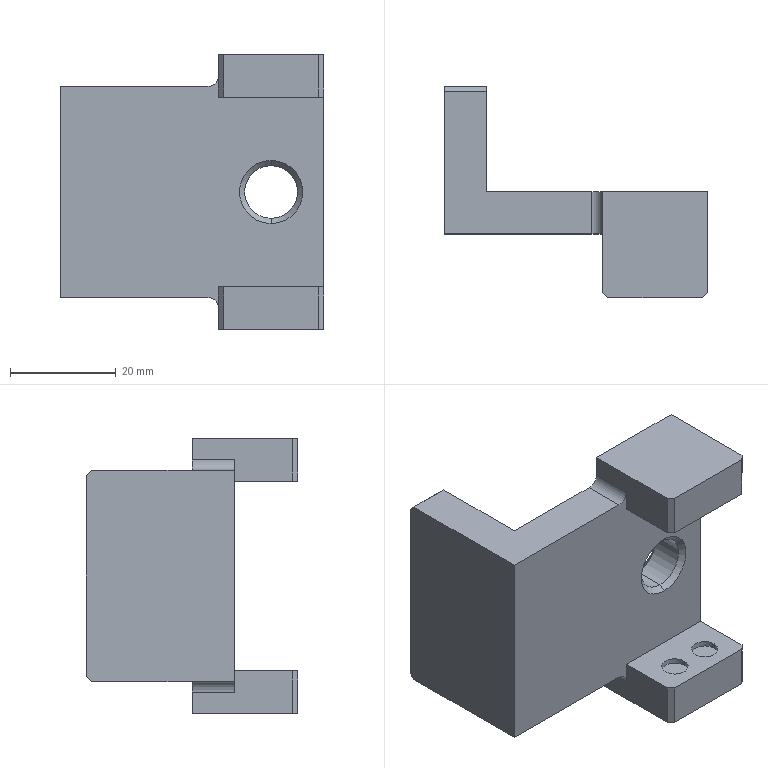Part | SolidWorks | features ICE 5, Chamfer 3, Cut 1, Extrusion 1, Fillet 1 | 1 solid | 42 faces | box 50 x 40 x 52 mm | volume 27409 mm3 | plane 26 | cylinder 12 | cone 4 | commonest cylinder face diameters 5 x8 4 x2 10 x2
STEP:
#1=CARTESIAN_POINT('',(38.5,-7.,39.));
#2=VERTEX_POINT('',#1);
#3=CARTESIAN_POINT('',(33.5,-7.,39.));
#4=VERTEX_POINT('',#3);
#5=CARTESIAN_POINT('',(36.,-7.,39.));
#6=DIRECTION('',(0.,0.,-1.));
#7=DIRECTION('',(-1.,0.,0.));
#8=AXIS2_PLACEMENT_3D('',#5,#6,#7);
#9=CIRCLE('',#8,2.5);
#10=EDGE_CURVE('',#2,#4,#9,.T.);
#11=ORIENTED_EDGE('',*,*,#10,.F.);
#12=CARTESIAN_POINT('',(38.5,-7.,38.));
#13=VERTEX_POINT('',#12);
#14=CARTESIAN_POINT('',(38.5,-7.,39.));
#15=DIRECTION('',(0.,0.,-1.));
#16=VECTOR('',#15,1000.);
#17=LINE('',#14,#16);
#18=EDGE_CURVE('',#2,#13,#17,.T.);
#19=ORIENTED_EDGE('',*,*,#18,.T.);
#20=CARTESIAN_POINT('',(33.5,-7.,38.));
#21=VERTEX_POINT('',#20);
#22=CARTESIAN_POINT('',(36.,-7.,38.));
#23=DIRECTION('',(0.,0.,-1.));
#24=DIRECTION('',(-1.,0.,0.));
#25=AXIS2_PLACEMENT_3D('',#22,#23,#24);
#26=CIRCLE('',#25,2.5);
#27=EDGE_CURVE('',#13,#21,#26,.T.);
#28=ORIENTED_EDGE('',*,*,#27,.T.);
#29=CARTESIAN_POINT('',(33.5,-7.,39.));
#30=DIRECTION('',(0.,0.,-1.));
#31=VECTOR('',#30,1000.);
#32=LINE('',#29,#31);
#33=EDGE_CURVE('',#4,#21,#32,.T.);
#34=ORIENTED_EDGE('',*,*,#33,.F.);
#35=EDGE_LOOP('',(#11,#19,#28,#34));
#36=FACE_OUTER_BOUND('',#35,.T.);
#37=CARTESIAN_POINT('',(36.,-7.,39.));
#38=DIRECTION('',(0.,0.,-1.));
#39=DIRECTION('',(-1.,0.,0.));
#40=AXIS2_PLACEMENT_3D('',#37,#38,#39);
#41=CYLINDRICAL_SURFACE('',#40,2.5);
#42=ADVANCED_FACE('',(#36),#41,.F.);
#43=CARTESIAN_POINT('',(46.5,-7.,39.));
#44=VERTEX_POINT('',#43);
#45=CARTESIAN_POINT('',(41.5,-7.,39.));
#46=VERTEX_POINT('',#45);
#47=CARTESIAN_POINT('',(44.,-7.,39.));
#48=DIRECTION('',(0.,0.,-1.));
#49=DIRECTION('',(-1.,0.,0.));
#50=AXIS2_PLACEMENT_3D('',#47,#48,#49);
#51=CIRCLE('',#50,2.5);
#52=EDGE_CURVE('',#44,#46,#51,.T.);
#53=ORIENTED_EDGE('',*,*,#52,.F.);
#54=CARTESIAN_POINT('',(46.5,-7.,38.));
#55=VERTEX_POINT('',#54);
#56=CARTESIAN_POINT('',(46.5,-7.,39.));
#57=DIRECTION('',(0.,0.,-1.));
#58=VECTOR('',#57,1000.);
#59=LINE('',#56,#58);
#60=EDGE_CURVE('',#44,#55,#59,.T.);
#61=ORIENTED_EDGE('',*,*,#60,.T.);
#62=CARTESIAN_POINT('',(41.5,-7.,38.));
#63=VERTEX_POINT('',#62);
#64=CARTESIAN_POINT('',(44.,-7.,38.));
#65=DIRECTION('',(0.,0.,-1.));
#66=DIRECTION('',(-1.,0.,0.));
#67=AXIS2_PLACEMENT_3D('',#64,#65,#66);
#68=CIRCLE('',#67,2.5);
#69=EDGE_CURVE('',#55,#63,#68,.T.);
#70=ORIENTED_EDGE('',*,*,#69,.T.);
#71=CARTESIAN_POINT('',(41.5,-7.,39.));
#72=DIRECTION('',(0.,0.,-1.));
#73=VECTOR('',#72,1000.);
#74=LINE('',#71,#73);
#75=EDGE_CURVE('',#46,#63,#74,.T.);
#76=ORIENTED_EDGE('',*,*,#75,.F.);
#77=EDGE_LOOP('',(#53,#61,#70,#76));
#78=FACE_OUTER_BOUND('',#77,.T.);
#79=CARTESIAN_POINT('',(44.,-7.,39.));
#80=DIRECTION('',(0.,0.,-1.));
#81=DIRECTION('',(-1.,0.,0.));
#82=AXIS2_PLACEMENT_3D('',#79,#80,#81);
#83=CYLINDRICAL_SURFACE('',#82,2.5);
#84=ADVANCED_FACE('',(#78),#83,.F.);
#85=CARTESIAN_POINT('',(41.5,-7.,1.));
#86=VERTEX_POINT('',#85);
#87=CARTESIAN_POINT('',(46.5,-7.,1.));
#88=VERTEX_POINT('',#87);
#89=CARTESIAN_POINT('',(44.,-7.,1.));
#90=DIRECTION('',(0.,0.,1.));
#91=DIRECTION('',(1.,0.,0.));
#92=AXIS2_PLACEMENT_3D('',#89,#90,#91);
#93=CIRCLE('',#92,2.5);
#94=EDGE_CURVE('',#86,#88,#93,.T.);
#95=ORIENTED_EDGE('',*,*,#94,.F.);
#96=CARTESIAN_POINT('',(41.5,-7.,2.));
#97=VERTEX_POINT('',#96);
#98=CARTESIAN_POINT('',(41.5,-7.,1.));
#99=DIRECTION('',(0.,0.,1.));
#100=VECTOR('',#99,1000.);
#101=LINE('',#98,#100);
#102=EDGE_CURVE('',#86,#97,#101,.T.);
#103=ORIENTED_EDGE('',*,*,#102,.T.);
#104=CARTESIAN_POINT('',(46.5,-7.,2.));
#105=VERTEX_POINT('',#104);
#106=CARTESIAN_POINT('',(44.,-7.,2.));
#107=DIRECTION('',(0.,0.,1.));
#108=DIRECTION('',(1.,0.,0.));
#109=AXIS2_PLACEMENT_3D('',#106,#107,#108);
#110=CIRCLE('',#109,2.5);
#111=EDGE_CURVE('',#97,#105,#110,.T.);
#112=ORIENTED_EDGE('',*,*,#111,.T.);
#113=CARTESIAN_POINT('',(46.5,-7.,1.));
#114=DIRECTION('',(0.,0.,1.));
#115=VECTOR('',#114,1000.);
#116=LINE('',#113,#115);
#117=EDGE_CURVE('',#88,#105,#116,.T.);
#118=ORIENTED_EDGE('',*,*,#117,.F.);
#119=EDGE_LOOP('',(#95,#103,#112,#118));
#120=FACE_OUTER_BOUND('',#119,.T.);
#121=CARTESIAN_POINT('',(44.,-7.,1.));
#122=DIRECTION('',(0.,0.,1.));
#123=DIRECTION('',(1.,0.,0.));
#124=AXIS2_PLACEMENT_3D('',#121,#122,#123);
#125=CYLINDRICAL_SURFACE('',#124,2.5);
#126=ADVANCED_FACE('',(#120),#125,.F.);
#127=CARTESIAN_POINT('',(33.5,-7.,1.));
#128=VERTEX_POINT('',#127);
#129=CARTESIAN_POINT('',(38.5,-7.,1.));
#130=VERTEX_POINT('',#129);
#131=CARTESIAN_POINT('',(36.,-7.,1.));
#132=DIRECTION('',(0.,0.,1.));
#133=DIRECTION('',(1.,0.,0.));
#134=AXIS2_PLACEMENT_3D('',#131,#132,#133);
#135=CIRCLE('',#134,2.5);
#136=EDGE_CURVE('',#128,#130,#135,.T.);
#137=ORIENTED_EDGE('',*,*,#136,.F.);
#138=CARTESIAN_POINT('',(33.5,-7.,2.));
#139=VERTEX_POINT('',#138);
#140=CARTESIAN_POINT('',(33.5,-7.,1.));
#141=DIRECTION('',(0.,0.,1.));
#142=VECTOR('',#141,1000.);
#143=LINE('',#140,#142);
#144=EDGE_CURVE('',#128,#139,#143,.T.);
#145=ORIENTED_EDGE('',*,*,#144,.T.);
#146=CARTESIAN_POINT('',(38.5,-7.,2.));
#147=VERTEX_POINT('',#146);
#148=CARTESIAN_POINT('',(36.,-7.,2.));
#149=DIRECTION('',(0.,0.,1.));
#150=DIRECTION('',(1.,0.,0.));
#151=AXIS2_PLACEMENT_3D('',#148,#149,#150);
#152=CIRCLE('',#151,2.5);
#153=EDGE_CURVE('',#139,#147,#152,.T.);
#154=ORIENTED_EDGE('',*,*,#153,.T.);
#155=CARTESIAN_POINT('',(38.5,-7.,1.));
#156=DIRECTION('',(0.,0.,1.));
#157=VECTOR('',#156,1000.);
#158=LINE('',#155,#157);
#159=EDGE_CURVE('',#130,#147,#158,.T.);
#160=ORIENTED_EDGE('',*,*,#159,.F.);
#161=EDGE_LOOP('',(#137,#145,#154,#160));
#162=FACE_OUTER_BOUND('',#161,.T.);
#163=CARTESIAN_POINT('',(36.,-7.,1.));
#164=DIRECTION('',(0.,0.,1.));
#165=DIRECTION('',(1.,0.,0.));
#166=AXIS2_PLACEMENT_3D('',#163,#164,#165);
#167=CYLINDRICAL_SURFACE('',#166,2.5);
#168=ADVANCED_FACE('',(#162),#167,.F.);
#169=CARTESIAN_POINT('',(40.,1.,25.));
#170=VERTEX_POINT('',#169);
#171=CARTESIAN_POINT('',(40.,1.,15.));
#172=VERTEX_POINT('',#171);
#173=CARTESIAN_POINT('',(40.,1.,20.));
#174=DIRECTION('',(0.,-1.,0.));
#175=DIRECTION('',(0.,0.,1.));
#176=AXIS2_PLACEMENT_3D('',#173,#174,#175);
#177=CIRCLE('',#176,5.);
#178=EDGE_CURVE('',#170,#172,#177,.T.);
#179=ORIENTED_EDGE('',*,*,#178,.F.);
#180=CARTESIAN_POINT('',(40.,0.,26.));
#181=VERTEX_POINT('',#180);
#182=CARTESIAN_POINT('',(40.,1.,25.));
#183=DIRECTION('',(0.,-0.7071,0.7071));
#184=VECTOR('',#183,1000.);
#185=LINE('',#182,#184);
#186=EDGE_CURVE('',#170,#181,#185,.T.);
#187=ORIENTED_EDGE('',*,*,#186,.T.);
#188=CARTESIAN_POINT('',(40.,0.,14.));
#189=VERTEX_POINT('',#188);
#190=CARTESIAN_POINT('',(40.,0.,20.));
#191=DIRECTION('',(0.,1.,0.));
#192=DIRECTION('',(0.,0.,1.));
#193=AXIS2_PLACEMENT_3D('',#190,#191,#192);
#194=CIRCLE('',#193,6.);
#195=EDGE_CURVE('',#189,#181,#194,.T.);
#196=ORIENTED_EDGE('',*,*,#195,.F.);
#197=CARTESIAN_POINT('',(40.,1.,15.));
#198=DIRECTION('',(0.,-0.7071,-0.7071));
#199=VECTOR('',#198,1000.);
#200=LINE('',#197,#199);
#201=EDGE_CURVE('',#172,#189,#200,.T.);
#202=ORIENTED_EDGE('',*,*,#201,.F.);
#203=EDGE_LOOP('',(#179,#187,#196,#202));
#204=FACE_OUTER_BOUND('',#203,.T.);
#205=CARTESIAN_POINT('',(40.,1.,20.));
#206=DIRECTION('',(0.,-1.,0.));
#207=DIRECTION('',(0.,0.,-1.));
#208=AXIS2_PLACEMENT_3D('',#205,#206,#207);
#209=CONICAL_SURFACE('',#208,5.,0.7854);
#210=ADVANCED_FACE('',(#204),#209,.F.);
#211=CARTESIAN_POINT('',(40.,7.,15.));
#212=VERTEX_POINT('',#211);
#213=CARTESIAN_POINT('',(40.,7.,25.));
#214=VERTEX_POINT('',#213);
#215=CARTESIAN_POINT('',(40.,7.,20.));
#216=DIRECTION('',(0.,1.,0.));
#217=DIRECTION('',(0.,0.,1.));
#218=AXIS2_PLACEMENT_3D('',#215,#216,#217);
#219=CIRCLE('',#218,5.);
#220=EDGE_CURVE('',#212,#214,#219,.T.);
#221=ORIENTED_EDGE('',*,*,#220,.F.);
#222=CARTESIAN_POINT('',(40.,8.,14.));
#223=VERTEX_POINT('',#222);
#224=CARTESIAN_POINT('',(40.,8.,14.));
#225=DIRECTION('',(0.,0.7071,-0.7071));
#226=VECTOR('',#225,1000.);
#227=LINE('',#224,#226);
#228=EDGE_CURVE('',#212,#223,#227,.T.);
#229=ORIENTED_EDGE('',*,*,#228,.T.);
#230=CARTESIAN_POINT('',(40.,8.,26.));
#231=VERTEX_POINT('',#230);
#232=CARTESIAN_POINT('',(40.,8.,20.));
#233=DIRECTION('',(0.,-1.,0.));
#234=DIRECTION('',(0.,0.,1.));
#235=AXIS2_PLACEMENT_3D('',#232,#233,#234);
#236=CIRCLE('',#235,6.);
#237=EDGE_CURVE('',#231,#223,#236,.T.);
#238=ORIENTED_EDGE('',*,*,#237,.F.);
#239=CARTESIAN_POINT('',(40.,8.,26.));
#240=DIRECTION('',(0.,0.7071,0.7071));
#241=VECTOR('',#240,1000.);
#242=LINE('',#239,#241);
#243=EDGE_CURVE('',#214,#231,#242,.T.);
#244=ORIENTED_EDGE('',*,*,#243,.F.);
#245=EDGE_LOOP('',(#221,#229,#238,#244));
#246=FACE_OUTER_BOUND('',#245,.T.);
#247=CARTESIAN_POINT('',(40.,8.,20.));
#248=DIRECTION('',(0.,1.,0.));
#249=DIRECTION('',(0.,0.,1.));
#250=AXIS2_PLACEMENT_3D('',#247,#248,#249);
#251=CONICAL_SURFACE('',#250,6.,0.7854);
#252=ADVANCED_FACE('',(#246),#251,.F.);
#253=ORIENTED_EDGE('',*,*,#220,.T.);
#254=CARTESIAN_POINT('',(40.,8.,25.));
#255=DIRECTION('',(0.,-1.,0.));
#256=VECTOR('',#255,1000.);
#257=LINE('',#254,#256);
#258=EDGE_CURVE('',#214,#170,#257,.T.);
#259=ORIENTED_EDGE('',*,*,#258,.T.);
#260=ORIENTED_EDGE('',*,*,#178,.T.);
#261=CARTESIAN_POINT('',(40.,8.,15.));
#262=DIRECTION('',(0.,-1.,0.));
#263=VECTOR('',#262,1000.);
#264=LINE('',#261,#263);
#265=EDGE_CURVE('',#212,#172,#264,.T.);
#266=ORIENTED_EDGE('',*,*,#265,.F.);
#267=EDGE_LOOP('',(#253,#259,#260,#266));
#268=FACE_OUTER_BOUND('',#267,.T.);
#269=CARTESIAN_POINT('',(40.,8.,20.));
#270=DIRECTION('',(0.,-1.,0.));
#271=DIRECTION('',(0.,0.,-1.));
#272=AXIS2_PLACEMENT_3D('',#269,#270,#271);
#273=CYLINDRICAL_SURFACE('',#272,5.);
#274=ADVANCED_FACE('',(#268),#273,.F.);
#275=CARTESIAN_POINT('',(0.,28.,1.));
#276=VERTEX_POINT('',#275);
#277=CARTESIAN_POINT('',(0.,28.,39.));
#278=VERTEX_POINT('',#277);
#279=CARTESIAN_POINT('',(0.,28.,0.));
#280=DIRECTION('',(0.,0.,1.));
#281=VECTOR('',#280,1000.);
#282=LINE('',#279,#281);
#283=EDGE_CURVE('',#276,#278,#282,.T.);
#284=ORIENTED_EDGE('',*,*,#283,.F.);
#285=CARTESIAN_POINT('',(0.,27.,0.));
#286=VERTEX_POINT('',#285);
#287=CARTESIAN_POINT('',(0.,28.,1.));
#288=DIRECTION('',(0.,-0.7071,-0.7071));
#289=VECTOR('',#288,1000.);
#290=LINE('',#287,#289);
#291=EDGE_CURVE('',#276,#286,#290,.T.);
#292=ORIENTED_EDGE('',*,*,#291,.T.);
#293=CARTESIAN_POINT('',(0.,0.,0.));
#294=VERTEX_POINT('',#293);
#295=CARTESIAN_POINT('',(0.,8.,0.));
#296=DIRECTION('',(0.,-1.,0.));
#297=VECTOR('',#296,1000.);
#298=LINE('',#295,#297);
#299=EDGE_CURVE('',#286,#294,#298,.T.);
#300=ORIENTED_EDGE('',*,*,#299,.T.);
#301=CARTESIAN_POINT('',(0.,0.,40.));
#302=VERTEX_POINT('',#301);
#303=CARTESIAN_POINT('',(0.,0.,0.));
#304=DIRECTION('',(0.,0.,1.));
#305=VECTOR('',#304,1000.);
#306=LINE('',#303,#305);
#307=EDGE_CURVE('',#294,#302,#306,.T.);
#308=ORIENTED_EDGE('',*,*,#307,.T.);
#309=CARTESIAN_POINT('',(0.,27.,40.));
#310=VERTEX_POINT('',#309);
#311=CARTESIAN_POINT('',(0.,8.,40.));
#312=DIRECTION('',(0.,-1.,0.));
#313=VECTOR('',#312,1000.);
#314=LINE('',#311,#313);
#315=EDGE_CURVE('',#310,#302,#314,.T.);
#316=ORIENTED_EDGE('',*,*,#315,.F.);
#317=CARTESIAN_POINT('',(0.,28.,39.));
#318=DIRECTION('',(0.,0.7071,-0.7071));
#319=VECTOR('',#318,1000.);
#320=LINE('',#317,#319);
#321=EDGE_CURVE('',#310,#278,#320,.T.);
#322=ORIENTED_EDGE('',*,*,#321,.T.);
#323=EDGE_LOOP('',(#284,#292,#300,#308,#316,#322));
#324=FACE_OUTER_BOUND('',#323,.T.);
#325=CARTESIAN_POINT('',(0.,8.,0.));
#326=DIRECTION('',(1.,0.,0.));
#327=DIRECTION('',(0.,0.,-1.));
#328=AXIS2_PLACEMENT_3D('',#325,#326,#327);
#329=PLANE('',#328);
#330=ADVANCED_FACE('',(#324),#329,.F.);
#331=CARTESIAN_POINT('',(8.,27.,40.));
#332=VERTEX_POINT('',#331);
#333=CARTESIAN_POINT('',(8.,8.,40.));
#334=VERTEX_POINT('',#333);
#335=CARTESIAN_POINT('',(8.,28.,40.));
#336=DIRECTION('',(0.,-1.,0.));
#337=VECTOR('',#336,1000.);
#338=LINE('',#335,#337);
#339=EDGE_CURVE('',#332,#334,#338,.T.);
#340=ORIENTED_EDGE('',*,*,#339,.F.);
#341=CARTESIAN_POINT('',(0.,27.,40.));
#342=DIRECTION('',(-1.,0.,0.));
#343=VECTOR('',#342,1000.);
#344=LINE('',#341,#343);
#345=EDGE_CURVE('',#332,#310,#344,.T.);
#346=ORIENTED_EDGE('',*,*,#345,.T.);
#347=ORIENTED_EDGE('',*,*,#315,.T.);
#348=CARTESIAN_POINT('',(28.,0.,40.));
#349=VERTEX_POINT('',#348);
#350=CARTESIAN_POINT('',(0.,0.,40.));
#351=DIRECTION('',(1.,0.,0.));
#352=VECTOR('',#351,1000.);
#353=LINE('',#350,#352);
#354=EDGE_CURVE('',#302,#349,#353,.T.);
#355=ORIENTED_EDGE('',*,*,#354,.T.);
#356=CARTESIAN_POINT('',(28.,8.,40.));
#357=VERTEX_POINT('',#356);
#358=CARTESIAN_POINT('',(28.,8.,40.));
#359=DIRECTION('',(0.,1.,0.));
#360=VECTOR('',#359,1000.);
#361=LINE('',#358,#360);
#362=EDGE_CURVE('',#349,#357,#361,.T.);
#363=ORIENTED_EDGE('',*,*,#362,.T.);
#364=CARTESIAN_POINT('',(0.,8.,40.));
#365=DIRECTION('',(1.,0.,0.));
#366=VECTOR('',#365,1000.);
#367=LINE('',#364,#366);
#368=EDGE_CURVE('',#334,#357,#367,.T.);
#369=ORIENTED_EDGE('',*,*,#368,.F.);
#370=EDGE_LOOP('',(#340,#346,#347,#355,#363,#369));
#371=FACE_OUTER_BOUND('',#370,.T.);
#372=CARTESIAN_POINT('',(0.,8.,40.));
#373=DIRECTION('',(0.,0.,-1.));
#374=DIRECTION('',(-1.,0.,0.));
#375=AXIS2_PLACEMENT_3D('',#372,#373,#374);
#376=PLANE('',#375);
#377=ADVANCED_FACE('',(#371),#376,.F.);
#378=CARTESIAN_POINT('',(50.,-11.,46.));
#379=VERTEX_POINT('',#378);
#380=CARTESIAN_POINT('',(50.,8.,46.));
#381=VERTEX_POINT('',#380);
#382=CARTESIAN_POINT('',(50.,-55.714,46.));
#383=DIRECTION('',(0.,1.,0.));
#384=VECTOR('',#383,1000.);
#385=LINE('',#382,#384);
#386=EDGE_CURVE('',#379,#381,#385,.T.);
#387=ORIENTED_EDGE('',*,*,#386,.F.);
#388=CARTESIAN_POINT('',(50.,-11.,38.));
#389=VERTEX_POINT('',#388);
#390=CARTESIAN_POINT('',(50.,-11.,38.));
#391=DIRECTION('',(0.,0.,-1.));
#392=VECTOR('',#391,1000.);
#393=LINE('',#390,#392);
#394=EDGE_CURVE('',#379,#389,#393,.T.);
#395=ORIENTED_EDGE('',*,*,#394,.T.);
#396=CARTESIAN_POINT('',(50.,0.,38.));
#397=VERTEX_POINT('',#396);
#398=CARTESIAN_POINT('',(50.,-12.,38.));
#399=DIRECTION('',(0.,1.,0.));
#400=VECTOR('',#399,1000.);
#401=LINE('',#398,#400);
#402=EDGE_CURVE('',#389,#397,#401,.T.);
#403=ORIENTED_EDGE('',*,*,#402,.T.);
#404=CARTESIAN_POINT('',(50.,0.,2.));
#405=VERTEX_POINT('',#404);
#406=CARTESIAN_POINT('',(50.,0.,0.));
#407=DIRECTION('',(0.,0.,-1.));
#408=VECTOR('',#407,1000.);
#409=LINE('',#406,#408);
#410=EDGE_CURVE('',#397,#405,#409,.T.);
#411=ORIENTED_EDGE('',*,*,#410,.T.);
#412=CARTESIAN_POINT('',(50.,-11.,2.));
#413=VERTEX_POINT('',#412);
#414=CARTESIAN_POINT('',(50.,-12.,2.));
#415=DIRECTION('',(0.,1.,0.));
#416=VECTOR('',#415,1000.);
#417=LINE('',#414,#416);
#418=EDGE_CURVE('',#413,#405,#417,.T.);
#419=ORIENTED_EDGE('',*,*,#418,.F.);
#420=CARTESIAN_POINT('',(50.,-11.,-6.));
#421=VERTEX_POINT('',#420);
#422=CARTESIAN_POINT('',(50.,-11.,0.));
#423=DIRECTION('',(0.,0.,-1.));
#424=VECTOR('',#423,1000.);
#425=LINE('',#422,#424);
#426=EDGE_CURVE('',#413,#421,#425,.T.);
#427=ORIENTED_EDGE('',*,*,#426,.T.);
#428=CARTESIAN_POINT('',(50.,8.,-6.));
#429=VERTEX_POINT('',#428);
#430=CARTESIAN_POINT('',(50.,-55.714,-6.));
#431=DIRECTION('',(0.,1.,0.));
#432=VECTOR('',#431,1000.);
#433=LINE('',#430,#432);
#434=EDGE_CURVE('',#421,#429,#433,.T.);
#435=ORIENTED_EDGE('',*,*,#434,.T.);
#436=CARTESIAN_POINT('',(50.,8.,0.));
#437=DIRECTION('',(0.,0.,-1.));
#438=VECTOR('',#437,1000.);
#439=LINE('',#436,#438);
#440=EDGE_CURVE('',#381,#429,#439,.T.);
#441=ORIENTED_EDGE('',*,*,#440,.F.);
#442=EDGE_LOOP('',(#387,#395,#403,#411,#419,#427,#435,#441));
#443=FACE_OUTER_BOUND('',#442,.T.);
#444=CARTESIAN_POINT('',(50.,8.,0.));
#445=DIRECTION('',(-1.,0.,0.));
#446=DIRECTION('',(0.,0.,1.));
#447=AXIS2_PLACEMENT_3D('',#444,#445,#446);
#448=PLANE('',#447);
#449=ADVANCED_FACE('',(#443),#448,.F.);
#450=ORIENTED_EDGE('',*,*,#299,.F.);
#451=CARTESIAN_POINT('',(8.,27.,0.));
#452=VERTEX_POINT('',#451);
#453=CARTESIAN_POINT('',(8.,27.,0.));
#454=DIRECTION('',(1.,0.,0.));
#455=VECTOR('',#454,1000.);
#456=LINE('',#453,#455);
#457=EDGE_CURVE('',#286,#452,#456,.T.);
#458=ORIENTED_EDGE('',*,*,#457,.T.);
#459=CARTESIAN_POINT('',(8.,8.,0.));
#460=VERTEX_POINT('',#459);
#461=CARTESIAN_POINT('',(8.,28.,0.));
#462=DIRECTION('',(0.,-1.,0.));
#463=VECTOR('',#462,1000.);
#464=LINE('',#461,#463);
#465=EDGE_CURVE('',#452,#460,#464,.T.);
#466=ORIENTED_EDGE('',*,*,#465,.T.);
#467=CARTESIAN_POINT('',(28.,8.,0.));
#468=VERTEX_POINT('',#467);
#469=CARTESIAN_POINT('',(0.,8.,0.));
#470=DIRECTION('',(-1.,0.,0.));
#471=VECTOR('',#470,1000.);
#472=LINE('',#469,#471);
#473=EDGE_CURVE('',#468,#460,#472,.T.);
#474=ORIENTED_EDGE('',*,*,#473,.F.);
#475=CARTESIAN_POINT('',(28.,0.,0.));
#476=VERTEX_POINT('',#475);
#477=CARTESIAN_POINT('',(28.,8.,0.));
#478=DIRECTION('',(0.,-1.,0.));
#479=VECTOR('',#478,1000.);
#480=LINE('',#477,#479);
#481=EDGE_CURVE('',#468,#476,#480,.T.);
#482=ORIENTED_EDGE('',*,*,#481,.T.);
#483=CARTESIAN_POINT('',(0.,0.,0.));
#484=DIRECTION('',(-1.,0.,0.));
#485=VECTOR('',#484,1000.);
#486=LINE('',#483,#485);
#487=EDGE_CURVE('',#476,#294,#486,.T.);
#488=ORIENTED_EDGE('',*,*,#487,.T.);
#489=EDGE_LOOP('',(#450,#458,#466,#474,#482,#488));
#490=FACE_OUTER_BOUND('',#489,.T.);
#491=CARTESIAN_POINT('',(0.,8.,0.));
#492=DIRECTION('',(0.,0.,1.));
#493=DIRECTION('',(1.,0.,0.));
#494=AXIS2_PLACEMENT_3D('',#491,#492,#493);
#495=PLANE('',#494);
#496=ADVANCED_FACE('',(#490),#495,.F.);
#497=CARTESIAN_POINT('',(8.,8.,0.));
#498=DIRECTION('',(0.,0.,-1.));
#499=VECTOR('',#498,1000.);
#500=LINE('',#497,#499);
#501=EDGE_CURVE('',#334,#460,#500,.T.);
#502=ORIENTED_EDGE('',*,*,#501,.F.);
#503=ORIENTED_EDGE('',*,*,#368,.T.);
#504=CARTESIAN_POINT('',(30.,8.,42.));
#505=VERTEX_POINT('',#504);
#506=CARTESIAN_POINT('',(28.,8.,42.));
#507=DIRECTION('',(0.,-1.,0.));
#508=DIRECTION('',(0.,0.,1.));
#509=AXIS2_PLACEMENT_3D('',#506,#507,#508);
#510=CIRCLE('',#509,2.);
#511=EDGE_CURVE('',#357,#505,#510,.T.);
#512=ORIENTED_EDGE('',*,*,#511,.T.);
#513=CARTESIAN_POINT('',(30.,8.,46.));
#514=VERTEX_POINT('',#513);
#515=CARTESIAN_POINT('',(30.,8.,-6.));
#516=DIRECTION('',(0.,0.,1.));
#517=VECTOR('',#516,1000.);
#518=LINE('',#515,#517);
#519=EDGE_CURVE('',#505,#514,#518,.T.);
#520=ORIENTED_EDGE('',*,*,#519,.T.);
#521=CARTESIAN_POINT('',(30.,8.,46.));
#522=DIRECTION('',(1.,0.,0.));
#523=VECTOR('',#522,1000.);
#524=LINE('',#521,#523);
#525=EDGE_CURVE('',#514,#381,#524,.T.);
#526=ORIENTED_EDGE('',*,*,#525,.T.);
#527=ORIENTED_EDGE('',*,*,#440,.T.);
#528=CARTESIAN_POINT('',(30.,8.,-6.));
#529=VERTEX_POINT('',#528);
#530=CARTESIAN_POINT('',(30.,8.,-6.));
#531=DIRECTION('',(-1.,0.,0.));
#532=VECTOR('',#531,1000.);
#533=LINE('',#530,#532);
#534=EDGE_CURVE('',#429,#529,#533,.T.);
#535=ORIENTED_EDGE('',*,*,#534,.T.);
#536=CARTESIAN_POINT('',(30.,8.,-2.));
#537=VERTEX_POINT('',#536);
#538=CARTESIAN_POINT('',(30.,8.,-6.));
#539=DIRECTION('',(0.,0.,1.));
#540=VECTOR('',#539,1000.);
#541=LINE('',#538,#540);
#542=EDGE_CURVE('',#529,#537,#541,.T.);
#543=ORIENTED_EDGE('',*,*,#542,.T.);
#544=CARTESIAN_POINT('',(28.,8.,-2.));
#545=DIRECTION('',(0.,-1.,0.));
#546=DIRECTION('',(0.,0.,1.));
#547=AXIS2_PLACEMENT_3D('',#544,#545,#546);
#548=CIRCLE('',#547,2.);
#549=EDGE_CURVE('',#537,#468,#548,.T.);
#550=ORIENTED_EDGE('',*,*,#549,.T.);
#551=ORIENTED_EDGE('',*,*,#473,.T.);
#552=EDGE_LOOP('',(#502,#503,#512,#520,#526,#527,#535,#543,#550,#551));
#553=FACE_OUTER_BOUND('',#552,.T.);
#554=ORIENTED_EDGE('',*,*,#237,.T.);
#555=CARTESIAN_POINT('',(40.,8.,20.));
#556=DIRECTION('',(0.,-1.,0.));
#557=DIRECTION('',(0.,0.,1.));
#558=AXIS2_PLACEMENT_3D('',#555,#556,#557);
#559=CIRCLE('',#558,6.);
#560=EDGE_CURVE('',#223,#231,#559,.T.);
#561=ORIENTED_EDGE('',*,*,#560,.T.);
#562=EDGE_LOOP('',(#554,#561));
#563=FACE_BOUND('',#562,.T.);
#564=CARTESIAN_POINT('',(0.,8.,0.));
#565=DIRECTION('',(0.,1.,0.));
#566=DIRECTION('',(0.,0.,1.));
#567=AXIS2_PLACEMENT_3D('',#564,#565,#566);
#568=PLANE('',#567);
#569=ADVANCED_FACE('',(#553,#563),#568,.T.);
#570=ORIENTED_EDGE('',*,*,#195,.T.);
#571=CARTESIAN_POINT('',(40.,0.,20.));
#572=DIRECTION('',(0.,1.,0.));
#573=DIRECTION('',(0.,0.,1.));
#574=AXIS2_PLACEMENT_3D('',#571,#572,#573);
#575=CIRCLE('',#574,6.);
#576=EDGE_CURVE('',#181,#189,#575,.T.);
#577=ORIENTED_EDGE('',*,*,#576,.T.);
#578=EDGE_LOOP('',(#570,#577));
#579=FACE_BOUND('',#578,.T.);
#580=ORIENTED_EDGE('',*,*,#487,.F.);
#581=CARTESIAN_POINT('',(30.,0.,-2.));
#582=VERTEX_POINT('',#581);
#583=CARTESIAN_POINT('',(28.,0.,-2.));
#584=DIRECTION('',(0.,1.,0.));
#585=DIRECTION('',(0.,0.,1.));
#586=AXIS2_PLACEMENT_3D('',#583,#584,#585);
#587=CIRCLE('',#586,2.);
#588=EDGE_CURVE('',#476,#582,#587,.T.);
#589=ORIENTED_EDGE('',*,*,#588,.T.);
#590=CARTESIAN_POINT('',(30.,0.,2.));
#591=VERTEX_POINT('',#590);
#592=CARTESIAN_POINT('',(30.,0.,-6.));
#593=DIRECTION('',(0.,0.,1.));
#594=VECTOR('',#593,1000.);
#595=LINE('',#592,#594);
#596=EDGE_CURVE('',#582,#591,#595,.T.);
#597=ORIENTED_EDGE('',*,*,#596,.T.);
#598=CARTESIAN_POINT('',(30.,0.,2.));
#599=DIRECTION('',(1.,0.,0.));
#600=VECTOR('',#599,1000.);
#601=LINE('',#598,#600);
#602=EDGE_CURVE('',#591,#405,#601,.T.);
#603=ORIENTED_EDGE('',*,*,#602,.T.);
#604=ORIENTED_EDGE('',*,*,#410,.F.);
#605=CARTESIAN_POINT('',(30.,0.,38.));
#606=VERTEX_POINT('',#605);
#607=CARTESIAN_POINT('',(30.,0.,38.));
#608=DIRECTION('',(-1.,0.,0.));
#609=VECTOR('',#608,1000.);
#610=LINE('',#607,#609);
#611=EDGE_CURVE('',#397,#606,#610,.T.);
#612=ORIENTED_EDGE('',*,*,#611,.T.);
#613=CARTESIAN_POINT('',(30.,0.,42.));
#614=VERTEX_POINT('',#613);
#615=CARTESIAN_POINT('',(30.,0.,46.));
#616=DIRECTION('',(0.,0.,1.));
#617=VECTOR('',#616,1000.);
#618=LINE('',#615,#617);
#619=EDGE_CURVE('',#606,#614,#618,.T.);
#620=ORIENTED_EDGE('',*,*,#619,.T.);
#621=CARTESIAN_POINT('',(28.,0.,42.));
#622=DIRECTION('',(0.,1.,0.));
#623=DIRECTION('',(0.,0.,1.));
#624=AXIS2_PLACEMENT_3D('',#621,#622,#623);
#625=CIRCLE('',#624,2.);
#626=EDGE_CURVE('',#614,#349,#625,.T.);
#627=ORIENTED_EDGE('',*,*,#626,.T.);
#628=ORIENTED_EDGE('',*,*,#354,.F.);
#629=ORIENTED_EDGE('',*,*,#307,.F.);
#630=EDGE_LOOP('',(#580,#589,#597,#603,#604,#612,#620,#627,#628,#629));
#631=FACE_OUTER_BOUND('',#630,.T.);
#632=CARTESIAN_POINT('',(0.,0.,0.));
#633=DIRECTION('',(0.,1.,0.));
#634=DIRECTION('',(0.,0.,1.));
#635=AXIS2_PLACEMENT_3D('',#632,#633,#634);
#636=PLANE('',#635);
#637=ADVANCED_FACE('',(#579,#631),#636,.F.);
#638=ORIENTED_EDGE('',*,*,#434,.F.);
#639=CARTESIAN_POINT('',(49.,-12.,-6.));
#640=VERTEX_POINT('',#639);
#641=CARTESIAN_POINT('',(17.643,-43.357,-6.));
#642=DIRECTION('',(-0.7071,-0.7071,0.));
#643=VECTOR('',#642,1000.);
#644=LINE('',#641,#643);
#645=EDGE_CURVE('',#421,#640,#644,.T.);
#646=ORIENTED_EDGE('',*,*,#645,.T.);
#647=CARTESIAN_POINT('',(31.,-12.,-6.));
#648=VERTEX_POINT('',#647);
#649=CARTESIAN_POINT('',(30.,-12.,-6.));
#650=DIRECTION('',(-1.,0.,0.));
#651=VECTOR('',#650,1000.);
#652=LINE('',#649,#651);
#653=EDGE_CURVE('',#640,#648,#652,.T.);
#654=ORIENTED_EDGE('',*,*,#653,.T.);
#655=CARTESIAN_POINT('',(30.,-11.,-6.));
#656=VERTEX_POINT('',#655);
#657=CARTESIAN_POINT('',(52.357,-33.357,-6.));
#658=DIRECTION('',(-0.7071,0.7071,0.));
#659=VECTOR('',#658,1000.);
#660=LINE('',#657,#659);
#661=EDGE_CURVE('',#648,#656,#660,.T.);
#662=ORIENTED_EDGE('',*,*,#661,.T.);
#663=CARTESIAN_POINT('',(30.,-55.714,-6.));
#664=DIRECTION('',(0.,1.,0.));
#665=VECTOR('',#664,1000.);
#666=LINE('',#663,#665);
#667=EDGE_CURVE('',#656,#529,#666,.T.);
#668=ORIENTED_EDGE('',*,*,#667,.T.);
#669=ORIENTED_EDGE('',*,*,#534,.F.);
#670=EDGE_LOOP('',(#638,#646,#654,#662,#668,#669));
#671=FACE_OUTER_BOUND('',#670,.T.);
#672=CARTESIAN_POINT('',(30.,-55.714,-6.));
#673=DIRECTION('',(0.,0.,-1.));
#674=DIRECTION('',(-1.,0.,0.));
#675=AXIS2_PLACEMENT_3D('',#672,#673,#674);
#676=PLANE('',#675);
#677=ADVANCED_FACE('',(#671),#676,.T.);
#678=ORIENTED_EDGE('',*,*,#596,.F.);
#679=CARTESIAN_POINT('',(30.,-55.714,-2.));
#680=DIRECTION('',(0.,1.,0.));
#681=VECTOR('',#680,1000.);
#682=LINE('',#679,#681);
#683=EDGE_CURVE('',#582,#537,#682,.T.);
#684=ORIENTED_EDGE('',*,*,#683,.T.);
#685=ORIENTED_EDGE('',*,*,#542,.F.);
#686=ORIENTED_EDGE('',*,*,#667,.F.);
#687=CARTESIAN_POINT('',(30.,-11.,2.));
#688=VERTEX_POINT('',#687);
#689=CARTESIAN_POINT('',(30.,-11.,2.));
#690=DIRECTION('',(0.,0.,1.));
#691=VECTOR('',#690,1000.);
#692=LINE('',#689,#691);
#693=EDGE_CURVE('',#656,#688,#692,.T.);
#694=ORIENTED_EDGE('',*,*,#693,.T.);
#695=CARTESIAN_POINT('',(30.,-12.,2.));
#696=DIRECTION('',(0.,1.,0.));
#697=VECTOR('',#696,1000.);
#698=LINE('',#695,#697);
#699=EDGE_CURVE('',#688,#591,#698,.T.);
#700=ORIENTED_EDGE('',*,*,#699,.T.);
#701=EDGE_LOOP('',(#678,#684,#685,#686,#694,#700));
#702=FACE_OUTER_BOUND('',#701,.T.);
#703=CARTESIAN_POINT('',(30.,-55.714,-6.));
#704=DIRECTION('',(-1.,0.,0.));
#705=DIRECTION('',(0.,0.,1.));
#706=AXIS2_PLACEMENT_3D('',#703,#704,#705);
#707=PLANE('',#706);
#708=ADVANCED_FACE('',(#702),#707,.T.);
#709=ORIENTED_EDGE('',*,*,#519,.F.);
#710=CARTESIAN_POINT('',(30.,-55.714,42.));
#711=DIRECTION('',(0.,-1.,0.));
#712=VECTOR('',#711,1000.);
#713=LINE('',#710,#712);
#714=EDGE_CURVE('',#505,#614,#713,.T.);
#715=ORIENTED_EDGE('',*,*,#714,.T.);
#716=ORIENTED_EDGE('',*,*,#619,.F.);
#717=CARTESIAN_POINT('',(30.,-11.,38.));
#718=VERTEX_POINT('',#717);
#719=CARTESIAN_POINT('',(30.,-12.,38.));
#720=DIRECTION('',(0.,1.,0.));
#721=VECTOR('',#720,1000.);
#722=LINE('',#719,#721);
#723=EDGE_CURVE('',#718,#606,#722,.T.);
#724=ORIENTED_EDGE('',*,*,#723,.F.);
#725=CARTESIAN_POINT('',(30.,-11.,46.));
#726=VERTEX_POINT('',#725);
#727=CARTESIAN_POINT('',(30.,-11.,-6.));
#728=DIRECTION('',(0.,0.,1.));
#729=VECTOR('',#728,1000.);
#730=LINE('',#727,#729);
#731=EDGE_CURVE('',#718,#726,#730,.T.);
#732=ORIENTED_EDGE('',*,*,#731,.T.);
#733=CARTESIAN_POINT('',(30.,-55.714,46.));
#734=DIRECTION('',(0.,1.,0.));
#735=VECTOR('',#734,1000.);
#736=LINE('',#733,#735);
#737=EDGE_CURVE('',#726,#514,#736,.T.);
#738=ORIENTED_EDGE('',*,*,#737,.T.);
#739=EDGE_LOOP('',(#709,#715,#716,#724,#732,#738));
#740=FACE_OUTER_BOUND('',#739,.T.);
#741=CARTESIAN_POINT('',(30.,-55.714,-6.));
#742=DIRECTION('',(-1.,0.,0.));
#743=DIRECTION('',(0.,0.,1.));
#744=AXIS2_PLACEMENT_3D('',#741,#742,#743);
#745=PLANE('',#744);
#746=ADVANCED_FACE('',(#740),#745,.T.);
#747=CARTESIAN_POINT('',(31.,-12.,46.));
#748=VERTEX_POINT('',#747);
#749=CARTESIAN_POINT('',(49.,-12.,46.));
#750=VERTEX_POINT('',#749);
#751=CARTESIAN_POINT('',(30.,-12.,46.));
#752=DIRECTION('',(1.,0.,0.));
#753=VECTOR('',#752,1000.);
#754=LINE('',#751,#753);
#755=EDGE_CURVE('',#748,#750,#754,.T.);
#756=ORIENTED_EDGE('',*,*,#755,.T.);
#757=CARTESIAN_POINT('',(17.643,-43.357,46.));
#758=DIRECTION('',(0.7071,0.7071,0.));
#759=VECTOR('',#758,1000.);
#760=LINE('',#757,#759);
#761=EDGE_CURVE('',#750,#379,#760,.T.);
#762=ORIENTED_EDGE('',*,*,#761,.T.);
#763=ORIENTED_EDGE('',*,*,#386,.T.);
#764=ORIENTED_EDGE('',*,*,#525,.F.);
#765=ORIENTED_EDGE('',*,*,#737,.F.);
#766=CARTESIAN_POINT('',(52.357,-33.357,46.));
#767=DIRECTION('',(0.7071,-0.7071,0.));
#768=VECTOR('',#767,1000.);
#769=LINE('',#766,#768);
#770=EDGE_CURVE('',#726,#748,#769,.T.);
#771=ORIENTED_EDGE('',*,*,#770,.T.);
#772=EDGE_LOOP('',(#756,#762,#763,#764,#765,#771));
#773=FACE_OUTER_BOUND('',#772,.T.);
#774=CARTESIAN_POINT('',(30.,-55.714,46.));
#775=DIRECTION('',(0.,0.,1.));
#776=DIRECTION('',(1.,0.,0.));
#777=AXIS2_PLACEMENT_3D('',#774,#775,#776);
#778=PLANE('',#777);
#779=ADVANCED_FACE('',(#773),#778,.T.);
#780=ORIENTED_EDGE('',*,*,#258,.F.);
#781=CARTESIAN_POINT('',(40.,7.,20.));
#782=DIRECTION('',(0.,1.,0.));
#783=DIRECTION('',(0.,0.,1.));
#784=AXIS2_PLACEMENT_3D('',#781,#782,#783);
#785=CIRCLE('',#784,5.);
#786=EDGE_CURVE('',#214,#212,#785,.T.);
#787=ORIENTED_EDGE('',*,*,#786,.T.);
#788=ORIENTED_EDGE('',*,*,#265,.T.);
#789=CARTESIAN_POINT('',(40.,1.,20.));
#790=DIRECTION('',(0.,-1.,0.));
#791=DIRECTION('',(0.,0.,1.));
#792=AXIS2_PLACEMENT_3D('',#789,#790,#791);
#793=CIRCLE('',#792,5.);
#794=EDGE_CURVE('',#172,#170,#793,.T.);
#795=ORIENTED_EDGE('',*,*,#794,.T.);
#796=EDGE_LOOP('',(#780,#787,#788,#795));
#797=FACE_OUTER_BOUND('',#796,.T.);
#798=CARTESIAN_POINT('',(40.,8.,20.));
#799=DIRECTION('',(0.,-1.,0.));
#800=DIRECTION('',(0.,0.,-1.));
#801=AXIS2_PLACEMENT_3D('',#798,#799,#800);
#802=CYLINDRICAL_SURFACE('',#801,5.);
#803=ADVANCED_FACE('',(#797),#802,.F.);
#804=ORIENTED_EDGE('',*,*,#228,.F.);
#805=ORIENTED_EDGE('',*,*,#786,.F.);
#806=ORIENTED_EDGE('',*,*,#243,.T.);
#807=ORIENTED_EDGE('',*,*,#560,.F.);
#808=EDGE_LOOP('',(#804,#805,#806,#807));
#809=FACE_OUTER_BOUND('',#808,.T.);
#810=CARTESIAN_POINT('',(40.,8.,20.));
#811=DIRECTION('',(0.,1.,0.));
#812=DIRECTION('',(0.,0.,1.));
#813=AXIS2_PLACEMENT_3D('',#810,#811,#812);
#814=CONICAL_SURFACE('',#813,6.,0.7854);
#815=ADVANCED_FACE('',(#809),#814,.F.);
#816=ORIENTED_EDGE('',*,*,#186,.F.);
#817=ORIENTED_EDGE('',*,*,#794,.F.);
#818=ORIENTED_EDGE('',*,*,#201,.T.);
#819=ORIENTED_EDGE('',*,*,#576,.F.);
#820=EDGE_LOOP('',(#816,#817,#818,#819));
#821=FACE_OUTER_BOUND('',#820,.T.);
#822=CARTESIAN_POINT('',(40.,1.,20.));
#823=DIRECTION('',(0.,-1.,0.));
#824=DIRECTION('',(0.,0.,-1.));
#825=AXIS2_PLACEMENT_3D('',#822,#823,#824);
#826=CONICAL_SURFACE('',#825,5.,0.7854);
#827=ADVANCED_FACE('',(#821),#826,.F.);
#828=CARTESIAN_POINT('',(36.,-7.,38.));
#829=DIRECTION('',(0.,0.,-1.));
#830=DIRECTION('',(-1.,0.,0.));
#831=AXIS2_PLACEMENT_3D('',#828,#829,#830);
#832=CIRCLE('',#831,2.5);
#833=EDGE_CURVE('',#21,#13,#832,.T.);
#834=ORIENTED_EDGE('',*,*,#833,.F.);
#835=ORIENTED_EDGE('',*,*,#27,.F.);
#836=EDGE_LOOP('',(#834,#835));
#837=FACE_BOUND('',#836,.T.);
#838=CARTESIAN_POINT('',(44.,-7.,38.));
#839=DIRECTION('',(0.,0.,-1.));
#840=DIRECTION('',(-1.,0.,0.));
#841=AXIS2_PLACEMENT_3D('',#838,#839,#840);
#842=CIRCLE('',#841,2.5);
#843=EDGE_CURVE('',#63,#55,#842,.T.);
#844=ORIENTED_EDGE('',*,*,#843,.F.);
#845=ORIENTED_EDGE('',*,*,#69,.F.);
#846=EDGE_LOOP('',(#844,#845));
#847=FACE_BOUND('',#846,.T.);
#848=ORIENTED_EDGE('',*,*,#402,.F.);
#849=CARTESIAN_POINT('',(49.,-12.,38.));
#850=VERTEX_POINT('',#849);
#851=CARTESIAN_POINT('',(39.5,-21.5,38.));
#852=DIRECTION('',(-0.7071,-0.7071,0.));
#853=VECTOR('',#852,1000.);
#854=LINE('',#851,#853);
#855=EDGE_CURVE('',#389,#850,#854,.T.);
#856=ORIENTED_EDGE('',*,*,#855,.T.);
#857=CARTESIAN_POINT('',(31.,-12.,38.));
#858=VERTEX_POINT('',#857);
#859=CARTESIAN_POINT('',(30.,-12.,38.));
#860=DIRECTION('',(-1.,0.,0.));
#861=VECTOR('',#860,1000.);
#862=LINE('',#859,#861);
#863=EDGE_CURVE('',#850,#858,#862,.T.);
#864=ORIENTED_EDGE('',*,*,#863,.T.);
#865=CARTESIAN_POINT('',(30.5,-11.5,38.));
#866=DIRECTION('',(-0.7071,0.7071,0.));
#867=VECTOR('',#866,1000.);
#868=LINE('',#865,#867);
#869=EDGE_CURVE('',#858,#718,#868,.T.);
#870=ORIENTED_EDGE('',*,*,#869,.T.);
#871=ORIENTED_EDGE('',*,*,#723,.T.);
#872=ORIENTED_EDGE('',*,*,#611,.F.);
#873=EDGE_LOOP('',(#848,#856,#864,#870,#871,#872));
#874=FACE_OUTER_BOUND('',#873,.T.);
#875=CARTESIAN_POINT('',(30.,-12.,38.));
#876=DIRECTION('',(0.,0.,-1.));
#877=DIRECTION('',(-1.,0.,0.));
#878=AXIS2_PLACEMENT_3D('',#875,#876,#877);
#879=PLANE('',#878);
#880=ADVANCED_FACE('',(#837,#847,#874),#879,.T.);
#881=ORIENTED_EDGE('',*,*,#863,.F.);
#882=CARTESIAN_POINT('',(49.,-12.,46.));
#883=DIRECTION('',(0.,0.,1.));
#884=VECTOR('',#883,1000.);
#885=LINE('',#882,#884);
#886=EDGE_CURVE('',#850,#750,#885,.T.);
#887=ORIENTED_EDGE('',*,*,#886,.T.);
#888=ORIENTED_EDGE('',*,*,#755,.F.);
#889=CARTESIAN_POINT('',(31.,-12.,0.));
#890=DIRECTION('',(0.,0.,-1.));
#891=VECTOR('',#890,1000.);
#892=LINE('',#889,#891);
#893=EDGE_CURVE('',#748,#858,#892,.T.);
#894=ORIENTED_EDGE('',*,*,#893,.T.);
#895=EDGE_LOOP('',(#881,#887,#888,#894));
#896=FACE_OUTER_BOUND('',#895,.T.);
#897=CARTESIAN_POINT('',(0.,-12.,0.));
#898=DIRECTION('',(0.,-1.,0.));
#899=DIRECTION('',(0.,0.,-1.));
#900=AXIS2_PLACEMENT_3D('',#897,#898,#899);
#901=PLANE('',#900);
#902=ADVANCED_FACE('',(#896),#901,.T.);
#903=CARTESIAN_POINT('',(44.,-7.,2.));
#904=DIRECTION('',(0.,0.,1.));
#905=DIRECTION('',(1.,0.,0.));
#906=AXIS2_PLACEMENT_3D('',#903,#904,#905);
#907=CIRCLE('',#906,2.5);
#908=EDGE_CURVE('',#105,#97,#907,.T.);
#909=ORIENTED_EDGE('',*,*,#908,.F.);
#910=ORIENTED_EDGE('',*,*,#111,.F.);
#911=EDGE_LOOP('',(#909,#910));
#912=FACE_BOUND('',#911,.T.);
#913=CARTESIAN_POINT('',(36.,-7.,2.));
#914=DIRECTION('',(0.,0.,1.));
#915=DIRECTION('',(1.,0.,0.));
#916=AXIS2_PLACEMENT_3D('',#913,#914,#915);
#917=CIRCLE('',#916,2.5);
#918=EDGE_CURVE('',#147,#139,#917,.T.);
#919=ORIENTED_EDGE('',*,*,#918,.F.);
#920=ORIENTED_EDGE('',*,*,#153,.F.);
#921=EDGE_LOOP('',(#919,#920));
#922=FACE_BOUND('',#921,.T.);
#923=CARTESIAN_POINT('',(31.,-12.,2.));
#924=VERTEX_POINT('',#923);
#925=CARTESIAN_POINT('',(49.,-12.,2.));
#926=VERTEX_POINT('',#925);
#927=CARTESIAN_POINT('',(30.,-12.,2.));
#928=DIRECTION('',(1.,0.,0.));
#929=VECTOR('',#928,1000.);
#930=LINE('',#927,#929);
#931=EDGE_CURVE('',#924,#926,#930,.T.);
#932=ORIENTED_EDGE('',*,*,#931,.T.);
#933=CARTESIAN_POINT('',(39.5,-21.5,2.));
#934=DIRECTION('',(0.7071,0.7071,0.));
#935=VECTOR('',#934,1000.);
#936=LINE('',#933,#935);
#937=EDGE_CURVE('',#926,#413,#936,.T.);
#938=ORIENTED_EDGE('',*,*,#937,.T.);
#939=ORIENTED_EDGE('',*,*,#418,.T.);
#940=ORIENTED_EDGE('',*,*,#602,.F.);
#941=ORIENTED_EDGE('',*,*,#699,.F.);
#942=CARTESIAN_POINT('',(30.5,-11.5,2.));
#943=DIRECTION('',(0.7071,-0.7071,0.));
#944=VECTOR('',#943,1000.);
#945=LINE('',#942,#944);
#946=EDGE_CURVE('',#688,#924,#945,.T.);
#947=ORIENTED_EDGE('',*,*,#946,.T.);
#948=EDGE_LOOP('',(#932,#938,#939,#940,#941,#947));
#949=FACE_OUTER_BOUND('',#948,.T.);
#950=CARTESIAN_POINT('',(30.,-12.,2.));
#951=DIRECTION('',(0.,0.,1.));
#952=DIRECTION('',(1.,0.,0.));
#953=AXIS2_PLACEMENT_3D('',#950,#951,#952);
#954=PLANE('',#953);
#955=ADVANCED_FACE('',(#912,#922,#949),#954,.T.);
#956=ORIENTED_EDGE('',*,*,#653,.F.);
#957=CARTESIAN_POINT('',(49.,-12.,0.));
#958=DIRECTION('',(0.,0.,1.));
#959=VECTOR('',#958,1000.);
#960=LINE('',#957,#959);
#961=EDGE_CURVE('',#640,#926,#960,.T.);
#962=ORIENTED_EDGE('',*,*,#961,.T.);
#963=ORIENTED_EDGE('',*,*,#931,.F.);
#964=CARTESIAN_POINT('',(31.,-12.,-6.));
#965=DIRECTION('',(0.,0.,-1.));
#966=VECTOR('',#965,1000.);
#967=LINE('',#964,#966);
#968=EDGE_CURVE('',#924,#648,#967,.T.);
#969=ORIENTED_EDGE('',*,*,#968,.T.);
#970=EDGE_LOOP('',(#956,#962,#963,#969));
#971=FACE_OUTER_BOUND('',#970,.T.);
#972=CARTESIAN_POINT('',(0.,-12.,0.));
#973=DIRECTION('',(0.,1.,0.));
#974=DIRECTION('',(0.,0.,1.));
#975=AXIS2_PLACEMENT_3D('',#972,#973,#974);
#976=PLANE('',#975);
#977=ADVANCED_FACE('',(#971),#976,.F.);
#978=ORIENTED_EDGE('',*,*,#761,.F.);
#979=ORIENTED_EDGE('',*,*,#886,.F.);
#980=ORIENTED_EDGE('',*,*,#855,.F.);
#981=ORIENTED_EDGE('',*,*,#394,.F.);
#982=EDGE_LOOP('',(#978,#979,#980,#981));
#983=FACE_OUTER_BOUND('',#982,.T.);
#984=CARTESIAN_POINT('',(50.,-11.,0.));
#985=DIRECTION('',(0.7071,-0.7071,0.));
#986=DIRECTION('',(0.,0.,1.));
#987=AXIS2_PLACEMENT_3D('',#984,#985,#986);
#988=PLANE('',#987);
#989=ADVANCED_FACE('',(#983),#988,.T.);
#990=ORIENTED_EDGE('',*,*,#869,.F.);
#991=ORIENTED_EDGE('',*,*,#893,.F.);
#992=ORIENTED_EDGE('',*,*,#770,.F.);
#993=ORIENTED_EDGE('',*,*,#731,.F.);
#994=EDGE_LOOP('',(#990,#991,#992,#993));
#995=FACE_OUTER_BOUND('',#994,.T.);
#996=CARTESIAN_POINT('',(30.,-11.,-6.));
#997=DIRECTION('',(0.7071,0.7071,0.));
#998=DIRECTION('',(0.,0.,1.));
#999=AXIS2_PLACEMENT_3D('',#996,#997,#998);
#1000=PLANE('',#999);
#1001=ADVANCED_FACE('',(#995),#1000,.F.);
#1002=ORIENTED_EDGE('',*,*,#937,.F.);
#1003=ORIENTED_EDGE('',*,*,#961,.F.);
#1004=ORIENTED_EDGE('',*,*,#645,.F.);
#1005=ORIENTED_EDGE('',*,*,#426,.F.);
#1006=EDGE_LOOP('',(#1002,#1003,#1004,#1005));
#1007=FACE_OUTER_BOUND('',#1006,.T.);
#1008=CARTESIAN_POINT('',(50.,-11.,0.));
#1009=DIRECTION('',(-0.7071,0.7071,0.));
#1010=DIRECTION('',(0.,0.,-1.));
#1011=AXIS2_PLACEMENT_3D('',#1008,#1009,#1010);
#1012=PLANE('',#1011);
#1013=ADVANCED_FACE('',(#1007),#1012,.F.);
#1014=ORIENTED_EDGE('',*,*,#661,.F.);
#1015=ORIENTED_EDGE('',*,*,#968,.F.);
#1016=ORIENTED_EDGE('',*,*,#946,.F.);
#1017=ORIENTED_EDGE('',*,*,#693,.F.);
#1018=EDGE_LOOP('',(#1014,#1015,#1016,#1017));
#1019=FACE_OUTER_BOUND('',#1018,.T.);
#1020=CARTESIAN_POINT('',(30.,-11.,-6.));
#1021=DIRECTION('',(-0.7071,-0.7071,0.));
#1022=DIRECTION('',(0.,0.,-1.));
#1023=AXIS2_PLACEMENT_3D('',#1020,#1021,#1022);
#1024=PLANE('',#1023);
#1025=ADVANCED_FACE('',(#1019),#1024,.T.);
#1026=ORIENTED_EDGE('',*,*,#626,.F.);
#1027=ORIENTED_EDGE('',*,*,#714,.F.);
#1028=ORIENTED_EDGE('',*,*,#511,.F.);
#1029=ORIENTED_EDGE('',*,*,#362,.F.);
#1030=EDGE_LOOP('',(#1026,#1027,#1028,#1029));
#1031=FACE_OUTER_BOUND('',#1030,.T.);
#1032=CARTESIAN_POINT('',(28.,8.,42.));
#1033=DIRECTION('',(0.,1.,0.));
#1034=DIRECTION('',(0.,0.,1.));
#1035=AXIS2_PLACEMENT_3D('',#1032,#1033,#1034);
#1036=CYLINDRICAL_SURFACE('',#1035,2.);
#1037=ADVANCED_FACE('',(#1031),#1036,.F.);
#1038=ORIENTED_EDGE('',*,*,#549,.F.);
#1039=ORIENTED_EDGE('',*,*,#683,.F.);
#1040=ORIENTED_EDGE('',*,*,#588,.F.);
#1041=ORIENTED_EDGE('',*,*,#481,.F.);
#1042=EDGE_LOOP('',(#1038,#1039,#1040,#1041));
#1043=FACE_OUTER_BOUND('',#1042,.T.);
#1044=CARTESIAN_POINT('',(28.,8.,-2.));
#1045=DIRECTION('',(0.,-1.,0.));
#1046=DIRECTION('',(0.,0.,-1.));
#1047=AXIS2_PLACEMENT_3D('',#1044,#1045,#1046);
#1048=CYLINDRICAL_SURFACE('',#1047,2.);
#1049=ADVANCED_FACE('',(#1043),#1048,.F.);
#1050=ORIENTED_EDGE('',*,*,#465,.F.);
#1051=CARTESIAN_POINT('',(8.,28.,1.));
#1052=VERTEX_POINT('',#1051);
#1053=CARTESIAN_POINT('',(8.,28.,1.));
#1054=DIRECTION('',(0.,0.7071,0.7071));
#1055=VECTOR('',#1054,1000.);
#1056=LINE('',#1053,#1055);
#1057=EDGE_CURVE('',#452,#1052,#1056,.T.);
#1058=ORIENTED_EDGE('',*,*,#1057,.T.);
#1059=CARTESIAN_POINT('',(8.,28.,39.));
#1060=VERTEX_POINT('',#1059);
#1061=CARTESIAN_POINT('',(8.,28.,0.));
#1062=DIRECTION('',(0.,0.,-1.));
#1063=VECTOR('',#1062,1000.);
#1064=LINE('',#1061,#1063);
#1065=EDGE_CURVE('',#1060,#1052,#1064,.T.);
#1066=ORIENTED_EDGE('',*,*,#1065,.F.);
#1067=CARTESIAN_POINT('',(8.,28.,39.));
#1068=DIRECTION('',(0.,-0.7071,0.7071));
#1069=VECTOR('',#1068,1000.);
#1070=LINE('',#1067,#1069);
#1071=EDGE_CURVE('',#1060,#332,#1070,.T.);
#1072=ORIENTED_EDGE('',*,*,#1071,.T.);
#1073=ORIENTED_EDGE('',*,*,#339,.T.);
#1074=ORIENTED_EDGE('',*,*,#501,.T.);
#1075=EDGE_LOOP('',(#1050,#1058,#1066,#1072,#1073,#1074));
#1076=FACE_OUTER_BOUND('',#1075,.T.);
#1077=CARTESIAN_POINT('',(8.,28.,0.));
#1078=DIRECTION('',(-1.,0.,0.));
#1079=DIRECTION('',(0.,0.,1.));
#1080=AXIS2_PLACEMENT_3D('',#1077,#1078,#1079);
#1081=PLANE('',#1080);
#1082=ADVANCED_FACE('',(#1076),#1081,.F.);
#1083=ORIENTED_EDGE('',*,*,#1065,.T.);
#1084=CARTESIAN_POINT('',(0.,28.,1.));
#1085=DIRECTION('',(-1.,0.,0.));
#1086=VECTOR('',#1085,1000.);
#1087=LINE('',#1084,#1086);
#1088=EDGE_CURVE('',#1052,#276,#1087,.T.);
#1089=ORIENTED_EDGE('',*,*,#1088,.T.);
#1090=ORIENTED_EDGE('',*,*,#283,.T.);
#1091=CARTESIAN_POINT('',(8.,28.,39.));
#1092=DIRECTION('',(1.,0.,0.));
#1093=VECTOR('',#1092,1000.);
#1094=LINE('',#1091,#1093);
#1095=EDGE_CURVE('',#278,#1060,#1094,.T.);
#1096=ORIENTED_EDGE('',*,*,#1095,.T.);
#1097=EDGE_LOOP('',(#1083,#1089,#1090,#1096));
#1098=FACE_OUTER_BOUND('',#1097,.T.);
#1099=CARTESIAN_POINT('',(0.,28.,0.));
#1100=DIRECTION('',(0.,1.,0.));
#1101=DIRECTION('',(0.,0.,1.));
#1102=AXIS2_PLACEMENT_3D('',#1099,#1100,#1101);
#1103=PLANE('',#1102);
#1104=ADVANCED_FACE('',(#1098),#1103,.T.);
#1105=ORIENTED_EDGE('',*,*,#1057,.F.);
#1106=ORIENTED_EDGE('',*,*,#457,.F.);
#1107=ORIENTED_EDGE('',*,*,#291,.F.);
#1108=ORIENTED_EDGE('',*,*,#1088,.F.);
#1109=EDGE_LOOP('',(#1105,#1106,#1107,#1108));
#1110=FACE_OUTER_BOUND('',#1109,.T.);
#1111=CARTESIAN_POINT('',(0.,28.,1.));
#1112=DIRECTION('',(0.,0.7071,-0.7071));
#1113=DIRECTION('',(1.,0.,0.));
#1114=AXIS2_PLACEMENT_3D('',#1111,#1112,#1113);
#1115=PLANE('',#1114);
#1116=ADVANCED_FACE('',(#1110),#1115,.T.);
#1117=ORIENTED_EDGE('',*,*,#321,.F.);
#1118=ORIENTED_EDGE('',*,*,#345,.F.);
#1119=ORIENTED_EDGE('',*,*,#1071,.F.);
#1120=ORIENTED_EDGE('',*,*,#1095,.F.);
#1121=EDGE_LOOP('',(#1117,#1118,#1119,#1120));
#1122=FACE_OUTER_BOUND('',#1121,.T.);
#1123=CARTESIAN_POINT('',(0.,28.,39.));
#1124=DIRECTION('',(0.,0.7071,0.7071));
#1125=DIRECTION('',(-1.,0.,0.));
#1126=AXIS2_PLACEMENT_3D('',#1123,#1124,#1125);
#1127=PLANE('',#1126);
#1128=ADVANCED_FACE('',(#1122),#1127,.T.);
#1129=ORIENTED_EDGE('',*,*,#144,.F.);
#1130=CARTESIAN_POINT('',(36.,-7.,1.));
#1131=DIRECTION('',(0.,0.,1.));
#1132=DIRECTION('',(1.,0.,0.));
#1133=AXIS2_PLACEMENT_3D('',#1130,#1131,#1132);
#1134=CIRCLE('',#1133,2.5);
#1135=EDGE_CURVE('',#130,#128,#1134,.T.);
#1136=ORIENTED_EDGE('',*,*,#1135,.F.);
#1137=ORIENTED_EDGE('',*,*,#159,.T.);
#1138=ORIENTED_EDGE('',*,*,#918,.T.);
#1139=EDGE_LOOP('',(#1129,#1136,#1137,#1138));
#1140=FACE_OUTER_BOUND('',#1139,.T.);
#1141=CARTESIAN_POINT('',(36.,-7.,1.));
#1142=DIRECTION('',(0.,0.,1.));
#1143=DIRECTION('',(1.,0.,0.));
#1144=AXIS2_PLACEMENT_3D('',#1141,#1142,#1143);
#1145=CYLINDRICAL_SURFACE('',#1144,2.5);
#1146=ADVANCED_FACE('',(#1140),#1145,.F.);
#1147=ORIENTED_EDGE('',*,*,#1135,.T.);
#1148=ORIENTED_EDGE('',*,*,#136,.T.);
#1149=EDGE_LOOP('',(#1147,#1148));
#1150=FACE_OUTER_BOUND('',#1149,.T.);
#1151=CARTESIAN_POINT('',(36.,-7.,1.));
#1152=DIRECTION('',(0.,0.,1.));
#1153=DIRECTION('',(1.,0.,0.));
#1154=AXIS2_PLACEMENT_3D('',#1151,#1152,#1153);
#1155=PLANE('',#1154);
#1156=ADVANCED_FACE('',(#1150),#1155,.T.);
#1157=ORIENTED_EDGE('',*,*,#102,.F.);
#1158=CARTESIAN_POINT('',(44.,-7.,1.));
#1159=DIRECTION('',(0.,0.,1.));
#1160=DIRECTION('',(1.,0.,0.));
#1161=AXIS2_PLACEMENT_3D('',#1158,#1159,#1160);
#1162=CIRCLE('',#1161,2.5);
#1163=EDGE_CURVE('',#88,#86,#1162,.T.);
#1164=ORIENTED_EDGE('',*,*,#1163,.F.);
#1165=ORIENTED_EDGE('',*,*,#117,.T.);
#1166=ORIENTED_EDGE('',*,*,#908,.T.);
#1167=EDGE_LOOP('',(#1157,#1164,#1165,#1166));
#1168=FACE_OUTER_BOUND('',#1167,.T.);
#1169=CARTESIAN_POINT('',(44.,-7.,1.));
#1170=DIRECTION('',(0.,0.,1.));
#1171=DIRECTION('',(1.,0.,0.));
#1172=AXIS2_PLACEMENT_3D('',#1169,#1170,#1171);
#1173=CYLINDRICAL_SURFACE('',#1172,2.5);
#1174=ADVANCED_FACE('',(#1168),#1173,.F.);
#1175=ORIENTED_EDGE('',*,*,#1163,.T.);
#1176=ORIENTED_EDGE('',*,*,#94,.T.);
#1177=EDGE_LOOP('',(#1175,#1176));
#1178=FACE_OUTER_BOUND('',#1177,.T.);
#1179=CARTESIAN_POINT('',(44.,-7.,1.));
#1180=DIRECTION('',(0.,0.,1.));
#1181=DIRECTION('',(1.,0.,0.));
#1182=AXIS2_PLACEMENT_3D('',#1179,#1180,#1181);
#1183=PLANE('',#1182);
#1184=ADVANCED_FACE('',(#1178),#1183,.T.);
#1185=ORIENTED_EDGE('',*,*,#60,.F.);
#1186=CARTESIAN_POINT('',(44.,-7.,39.));
#1187=DIRECTION('',(0.,0.,-1.));
#1188=DIRECTION('',(-1.,0.,0.));
#1189=AXIS2_PLACEMENT_3D('',#1186,#1187,#1188);
#1190=CIRCLE('',#1189,2.5);
#1191=EDGE_CURVE('',#46,#44,#1190,.T.);
#1192=ORIENTED_EDGE('',*,*,#1191,.F.);
#1193=ORIENTED_EDGE('',*,*,#75,.T.);
#1194=ORIENTED_EDGE('',*,*,#843,.T.);
#1195=EDGE_LOOP('',(#1185,#1192,#1193,#1194));
#1196=FACE_OUTER_BOUND('',#1195,.T.);
#1197=CARTESIAN_POINT('',(44.,-7.,39.));
#1198=DIRECTION('',(0.,0.,-1.));
#1199=DIRECTION('',(-1.,0.,0.));
#1200=AXIS2_PLACEMENT_3D('',#1197,#1198,#1199);
#1201=CYLINDRICAL_SURFACE('',#1200,2.5);
#1202=ADVANCED_FACE('',(#1196),#1201,.F.);
#1203=ORIENTED_EDGE('',*,*,#1191,.T.);
#1204=ORIENTED_EDGE('',*,*,#52,.T.);
#1205=EDGE_LOOP('',(#1203,#1204));
#1206=FACE_OUTER_BOUND('',#1205,.T.);
#1207=CARTESIAN_POINT('',(44.,-7.,39.));
#1208=DIRECTION('',(0.,0.,-1.));
#1209=DIRECTION('',(-1.,0.,0.));
#1210=AXIS2_PLACEMENT_3D('',#1207,#1208,#1209);
#1211=PLANE('',#1210);
#1212=ADVANCED_FACE('',(#1206),#1211,.T.);
#1213=ORIENTED_EDGE('',*,*,#18,.F.);
#1214=CARTESIAN_POINT('',(36.,-7.,39.));
#1215=DIRECTION('',(0.,0.,-1.));
#1216=DIRECTION('',(-1.,0.,0.));
#1217=AXIS2_PLACEMENT_3D('',#1214,#1215,#1216);
#1218=CIRCLE('',#1217,2.5);
#1219=EDGE_CURVE('',#4,#2,#1218,.T.);
#1220=ORIENTED_EDGE('',*,*,#1219,.F.);
#1221=ORIENTED_EDGE('',*,*,#33,.T.);
#1222=ORIENTED_EDGE('',*,*,#833,.T.);
#1223=EDGE_LOOP('',(#1213,#1220,#1221,#1222));
#1224=FACE_OUTER_BOUND('',#1223,.T.);
#1225=CARTESIAN_POINT('',(36.,-7.,39.));
#1226=DIRECTION('',(0.,0.,-1.));
#1227=DIRECTION('',(-1.,0.,0.));
#1228=AXIS2_PLACEMENT_3D('',#1225,#1226,#1227);
#1229=CYLINDRICAL_SURFACE('',#1228,2.5);
#1230=ADVANCED_FACE('',(#1224),#1229,.F.);
#1231=ORIENTED_EDGE('',*,*,#1219,.T.);
#1232=ORIENTED_EDGE('',*,*,#10,.T.);
#1233=EDGE_LOOP('',(#1231,#1232));
#1234=FACE_OUTER_BOUND('',#1233,.T.);
#1235=CARTESIAN_POINT('',(36.,-7.,39.));
#1236=DIRECTION('',(0.,0.,-1.));
#1237=DIRECTION('',(-1.,0.,0.));
#1238=AXIS2_PLACEMENT_3D('',#1235,#1236,#1237);
#1239=PLANE('',#1238);
#1240=ADVANCED_FACE('',(#1234),#1239,.T.);
#1241=CLOSED_SHELL('',(#42,#84,#126,#168,#210,#252,#274,#330,#377,#449,#496,#569,#637,#677,#708,#746,#779,#803,#815,#827,#880,#902,#955,#977,#989,#1001,#1013,#1025,#1037,#1049,#1082,#1104,#1116,#1128,#1146,#1156,#1174,#1184,#1202,#1212,#1230,#1240));
#1242=MANIFOLD_SOLID_BREP('',#1241);
#1243=CARTESIAN_POINT('',(0.,0.,0.));
#1244=DIRECTION('',(0.,0.,1.));
#1245=DIRECTION('',(1.,0.,0.));
#1246=AXIS2_PLACEMENT_3D('',#1243,#1244,#1245);
#1247=(LENGTH_UNIT()NAMED_UNIT(*)SI_UNIT(.MILLI.,.METRE.));
#1248=UNCERTAINTY_MEASURE_WITH_UNIT(LENGTH_MEASURE(0.00001),#1247,'','');
#1249=(NAMED_UNIT(*)PLANE_ANGLE_UNIT()SI_UNIT($,.RADIAN.));
#1250=(NAMED_UNIT(*)SI_UNIT($,.STERADIAN.)SOLID_ANGLE_UNIT());
#1251=(GEOMETRIC_REPRESENTATION_CONTEXT(3)GLOBAL_UNCERTAINTY_ASSIGNED_CONTEXT((#1248))GLOBAL_UNIT_ASSIGNED_CONTEXT((#1247,#1249,#1250))REPRESENTATION_CONTEXT('',''));
#1252=ADVANCED_BREP_SHAPE_REPRESENTATION('',(#1242,#1246),#1251);